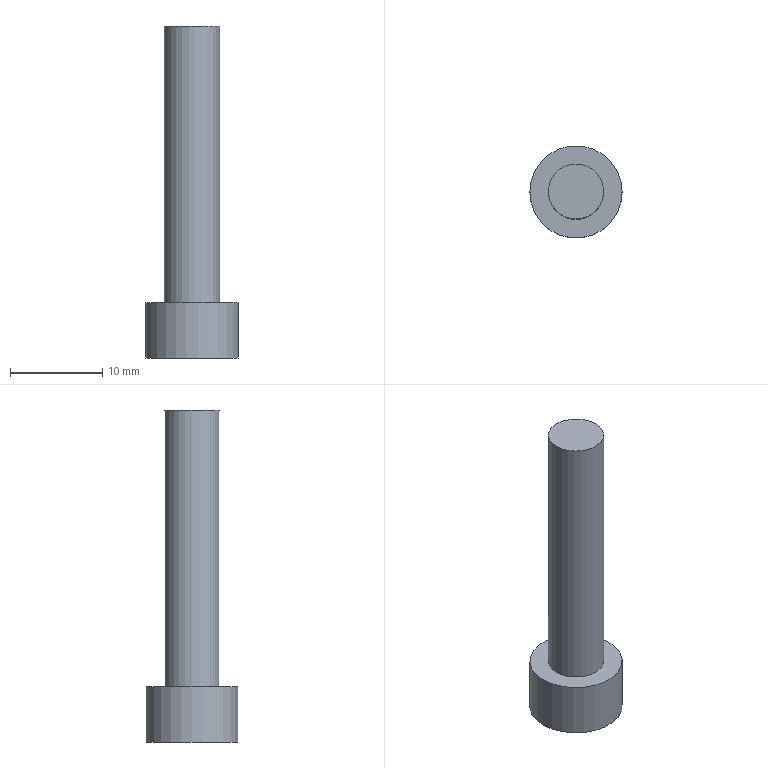Part | STEP file | 1 solid | 12 faces | box 10 x 10 x 36 mm | volume 1234 mm3 | plane 10 | cylinder 2 | commonest cylinder face diameters 6 x1 10 x1
STEP:
#1=CARTESIAN_POINT('',(0.,0.,0.));
#2=DIRECTION('',(0.,0.,1.));
#3=DIRECTION('',(1.,0.,0.));
#4=AXIS2_PLACEMENT_3D('',#1,#2,#3);
#5=CARTESIAN_POINT('',(1725.957,344.98,-64.381));
#6=VERTEX_POINT('',#5);
#7=CARTESIAN_POINT('',(1720.957,344.98,-64.381));
#8=DIRECTION('',(0.,0.,-1.));
#9=DIRECTION('',(1.,0.,0.));
#10=AXIS2_PLACEMENT_3D('',#7,#8,#9);
#11=CIRCLE('',#10,5.);
#12=CARTESIAN_POINT('',(1725.957,344.98,-64.381));
#13=DIRECTION('',(0.,0.,1.));
#14=DIRECTION('',(-1.,0.,0.));
#15=AXIS2_PLACEMENT_3D('',#12,#13,#14);
#16=PLANE('',#15);
#17=CARTESIAN_POINT('',(0.,0.));
#18=CARTESIAN_POINT('',(0.,8.66));
#19=CARTESIAN_POINT('',(7.5,4.33));
#20=CARTESIAN_POINT('',(15.,0.));
#21=CARTESIAN_POINT('',(7.5,-4.33));
#22=CARTESIAN_POINT('',(0.,-8.66));
#23=CARTESIAN_POINT('',(0.,0.));
#24=(BOUNDED_CURVE()B_SPLINE_CURVE(2,(#17,#18,#19,#20,#21,#22,#23),.UNSPECIFIED.,.T.,.F.)B_SPLINE_CURVE_WITH_KNOTS((1,2,2,2,2,1),(-2.094,0.,2.094,4.189,6.283,8.378),.UNSPECIFIED.)CURVE()GEOMETRIC_REPRESENTATION_ITEM()RATIONAL_B_SPLINE_CURVE((1.,0.5,1.,0.5,1.,0.5,1.))REPRESENTATION_ITEM(''));
#25=(GEOMETRIC_REPRESENTATION_CONTEXT(2)PARAMETRIC_REPRESENTATION_CONTEXT()REPRESENTATION_CONTEXT('',''));
#26=DEFINITIONAL_REPRESENTATION('',(#24),#25);
#27=PCURVE('',#16,#26);
#28=CARTESIAN_POINT('',(1720.957,344.98,-58.481));
#29=DIRECTION('',(0.,0.,-1.));
#30=DIRECTION('',(1.,0.,0.));
#31=AXIS2_PLACEMENT_3D('',#28,#29,#30);
#32=CYLINDRICAL_SURFACE('',#31,5.);
#33=CARTESIAN_POINT('',(0.,5.9));
#34=DIRECTION('',(1.,0.));
#35=VECTOR('',#34,1.);
#36=LINE('',#33,#35);
#37=(GEOMETRIC_REPRESENTATION_CONTEXT(2)PARAMETRIC_REPRESENTATION_CONTEXT()REPRESENTATION_CONTEXT('',''));
#38=DEFINITIONAL_REPRESENTATION('',(#36),#37);
#39=PCURVE('',#32,#38);
#40=SURFACE_CURVE('',#11,(#27,#39),.PCURVE_S1.);
#41=EDGE_CURVE('',#6,#6,#40,.T.);
#42=ORIENTED_EDGE('',*,*,#41,.T.);
#43=EDGE_LOOP('',(#42));
#44=FACE_BOUND('',#43,.T.);
#45=CARTESIAN_POINT('',(1719.514,342.48,-64.381));
#46=VERTEX_POINT('',#45);
#47=CARTESIAN_POINT('',(1722.401,342.48,-64.381));
#48=VERTEX_POINT('',#47);
#49=CARTESIAN_POINT('',(1719.514,342.48,-64.381));
#50=DIRECTION('',(1.,0.,0.));
#51=VECTOR('',#50,1.);
#52=LINE('',#49,#51);
#53=CARTESIAN_POINT('',(6.443,2.5));
#54=DIRECTION('',(-1.,0.));
#55=VECTOR('',#54,1.);
#56=LINE('',#53,#55);
#57=(GEOMETRIC_REPRESENTATION_CONTEXT(2)PARAMETRIC_REPRESENTATION_CONTEXT()REPRESENTATION_CONTEXT('',''));
#58=DEFINITIONAL_REPRESENTATION('',(#56),#57);
#59=PCURVE('',#16,#58);
#60=CARTESIAN_POINT('',(1719.514,342.48,-60.421));
#61=DIRECTION('',(0.,1.,0.));
#62=DIRECTION('',(1.,0.,0.));
#63=AXIS2_PLACEMENT_3D('',#60,#61,#62);
#64=PLANE('',#63);
#65=CARTESIAN_POINT('',(0.,3.96));
#66=DIRECTION('',(1.,0.));
#67=VECTOR('',#66,1.);
#68=LINE('',#65,#67);
#69=(GEOMETRIC_REPRESENTATION_CONTEXT(2)PARAMETRIC_REPRESENTATION_CONTEXT()REPRESENTATION_CONTEXT('',''));
#70=DEFINITIONAL_REPRESENTATION('',(#68),#69);
#71=PCURVE('',#64,#70);
#72=SURFACE_CURVE('',#52,(#59,#71),.PCURVE_S1.);
#73=EDGE_CURVE('',#46,#48,#72,.T.);
#74=ORIENTED_EDGE('',*,*,#73,.T.);
#75=CARTESIAN_POINT('',(1723.844,344.98,-64.381));
#76=VERTEX_POINT('',#75);
#77=CARTESIAN_POINT('',(1722.401,342.48,-64.381));
#78=DIRECTION('',(0.5,0.866,0.));
#79=VECTOR('',#78,1.);
#80=LINE('',#77,#79);
#81=CARTESIAN_POINT('',(3.557,2.5));
#82=DIRECTION('',(-0.5,-0.866));
#83=VECTOR('',#82,1.);
#84=LINE('',#81,#83);
#85=(GEOMETRIC_REPRESENTATION_CONTEXT(2)PARAMETRIC_REPRESENTATION_CONTEXT()REPRESENTATION_CONTEXT('',''));
#86=DEFINITIONAL_REPRESENTATION('',(#84),#85);
#87=PCURVE('',#16,#86);
#88=CARTESIAN_POINT('',(1722.401,342.48,-60.421));
#89=DIRECTION('',(-0.866,0.5,0.));
#90=DIRECTION('',(0.5,0.866,0.));
#91=AXIS2_PLACEMENT_3D('',#88,#89,#90);
#92=PLANE('',#91);
#93=CARTESIAN_POINT('',(0.,3.96));
#94=DIRECTION('',(1.,0.));
#95=VECTOR('',#94,1.);
#96=LINE('',#93,#95);
#97=(GEOMETRIC_REPRESENTATION_CONTEXT(2)PARAMETRIC_REPRESENTATION_CONTEXT()REPRESENTATION_CONTEXT('',''));
#98=DEFINITIONAL_REPRESENTATION('',(#96),#97);
#99=PCURVE('',#92,#98);
#100=SURFACE_CURVE('',#80,(#87,#99),.PCURVE_S1.);
#101=EDGE_CURVE('',#48,#76,#100,.T.);
#102=ORIENTED_EDGE('',*,*,#101,.T.);
#103=CARTESIAN_POINT('',(1722.401,347.48,-64.381));
#104=VERTEX_POINT('',#103);
#105=CARTESIAN_POINT('',(1723.844,344.98,-64.381));
#106=DIRECTION('',(-0.5,0.866,0.));
#107=VECTOR('',#106,1.);
#108=LINE('',#105,#107);
#109=CARTESIAN_POINT('',(2.113,0.));
#110=DIRECTION('',(0.5,-0.866));
#111=VECTOR('',#110,1.);
#112=LINE('',#109,#111);
#113=(GEOMETRIC_REPRESENTATION_CONTEXT(2)PARAMETRIC_REPRESENTATION_CONTEXT()REPRESENTATION_CONTEXT('',''));
#114=DEFINITIONAL_REPRESENTATION('',(#112),#113);
#115=PCURVE('',#16,#114);
#116=CARTESIAN_POINT('',(1723.844,344.98,-60.421));
#117=DIRECTION('',(-0.866,-0.5,0.));
#118=DIRECTION('',(-0.5,0.866,0.));
#119=AXIS2_PLACEMENT_3D('',#116,#117,#118);
#120=PLANE('',#119);
#121=CARTESIAN_POINT('',(0.,3.96));
#122=DIRECTION('',(1.,0.));
#123=VECTOR('',#122,1.);
#124=LINE('',#121,#123);
#125=(GEOMETRIC_REPRESENTATION_CONTEXT(2)PARAMETRIC_REPRESENTATION_CONTEXT()REPRESENTATION_CONTEXT('',''));
#126=DEFINITIONAL_REPRESENTATION('',(#124),#125);
#127=PCURVE('',#120,#126);
#128=SURFACE_CURVE('',#108,(#115,#127),.PCURVE_S1.);
#129=EDGE_CURVE('',#76,#104,#128,.T.);
#130=ORIENTED_EDGE('',*,*,#129,.T.);
#131=CARTESIAN_POINT('',(1719.514,347.48,-64.381));
#132=VERTEX_POINT('',#131);
#133=CARTESIAN_POINT('',(1722.401,347.48,-64.381));
#134=DIRECTION('',(-1.,0.,0.));
#135=VECTOR('',#134,1.);
#136=LINE('',#133,#135);
#137=CARTESIAN_POINT('',(3.557,-2.5));
#138=DIRECTION('',(1.,0.));
#139=VECTOR('',#138,1.);
#140=LINE('',#137,#139);
#141=(GEOMETRIC_REPRESENTATION_CONTEXT(2)PARAMETRIC_REPRESENTATION_CONTEXT()REPRESENTATION_CONTEXT('',''));
#142=DEFINITIONAL_REPRESENTATION('',(#140),#141);
#143=PCURVE('',#16,#142);
#144=CARTESIAN_POINT('',(1722.401,347.48,-60.421));
#145=DIRECTION('',(0.,-1.,0.));
#146=DIRECTION('',(-1.,0.,0.));
#147=AXIS2_PLACEMENT_3D('',#144,#145,#146);
#148=PLANE('',#147);
#149=CARTESIAN_POINT('',(0.,3.96));
#150=DIRECTION('',(1.,0.));
#151=VECTOR('',#150,1.);
#152=LINE('',#149,#151);
#153=(GEOMETRIC_REPRESENTATION_CONTEXT(2)PARAMETRIC_REPRESENTATION_CONTEXT()REPRESENTATION_CONTEXT('',''));
#154=DEFINITIONAL_REPRESENTATION('',(#152),#153);
#155=PCURVE('',#148,#154);
#156=SURFACE_CURVE('',#136,(#143,#155),.PCURVE_S1.);
#157=EDGE_CURVE('',#104,#132,#156,.T.);
#158=ORIENTED_EDGE('',*,*,#157,.T.);
#159=CARTESIAN_POINT('',(1718.07,344.98,-64.381));
#160=VERTEX_POINT('',#159);
#161=CARTESIAN_POINT('',(1719.514,347.48,-64.381));
#162=DIRECTION('',(-0.5,-0.866,0.));
#163=VECTOR('',#162,1.);
#164=LINE('',#161,#163);
#165=CARTESIAN_POINT('',(6.443,-2.5));
#166=DIRECTION('',(0.5,0.866));
#167=VECTOR('',#166,1.);
#168=LINE('',#165,#167);
#169=(GEOMETRIC_REPRESENTATION_CONTEXT(2)PARAMETRIC_REPRESENTATION_CONTEXT()REPRESENTATION_CONTEXT('',''));
#170=DEFINITIONAL_REPRESENTATION('',(#168),#169);
#171=PCURVE('',#16,#170);
#172=CARTESIAN_POINT('',(1719.514,347.48,-60.421));
#173=DIRECTION('',(0.866,-0.5,0.));
#174=DIRECTION('',(-0.5,-0.866,0.));
#175=AXIS2_PLACEMENT_3D('',#172,#173,#174);
#176=PLANE('',#175);
#177=CARTESIAN_POINT('',(0.,3.96));
#178=DIRECTION('',(1.,0.));
#179=VECTOR('',#178,1.);
#180=LINE('',#177,#179);
#181=(GEOMETRIC_REPRESENTATION_CONTEXT(2)PARAMETRIC_REPRESENTATION_CONTEXT()REPRESENTATION_CONTEXT('',''));
#182=DEFINITIONAL_REPRESENTATION('',(#180),#181);
#183=PCURVE('',#176,#182);
#184=SURFACE_CURVE('',#164,(#171,#183),.PCURVE_S1.);
#185=EDGE_CURVE('',#132,#160,#184,.T.);
#186=ORIENTED_EDGE('',*,*,#185,.T.);
#187=CARTESIAN_POINT('',(1718.07,344.98,-64.381));
#188=DIRECTION('',(0.5,-0.866,0.));
#189=VECTOR('',#188,1.);
#190=LINE('',#187,#189);
#191=CARTESIAN_POINT('',(7.887,0.));
#192=DIRECTION('',(-0.5,0.866));
#193=VECTOR('',#192,1.);
#194=LINE('',#191,#193);
#195=(GEOMETRIC_REPRESENTATION_CONTEXT(2)PARAMETRIC_REPRESENTATION_CONTEXT()REPRESENTATION_CONTEXT('',''));
#196=DEFINITIONAL_REPRESENTATION('',(#194),#195);
#197=PCURVE('',#16,#196);
#198=CARTESIAN_POINT('',(1718.07,344.98,-60.421));
#199=DIRECTION('',(0.866,0.5,0.));
#200=DIRECTION('',(0.5,-0.866,0.));
#201=AXIS2_PLACEMENT_3D('',#198,#199,#200);
#202=PLANE('',#201);
#203=CARTESIAN_POINT('',(0.,3.96));
#204=DIRECTION('',(1.,0.));
#205=VECTOR('',#204,1.);
#206=LINE('',#203,#205);
#207=(GEOMETRIC_REPRESENTATION_CONTEXT(2)PARAMETRIC_REPRESENTATION_CONTEXT()REPRESENTATION_CONTEXT('',''));
#208=DEFINITIONAL_REPRESENTATION('',(#206),#207);
#209=PCURVE('',#202,#208);
#210=SURFACE_CURVE('',#190,(#197,#209),.PCURVE_S1.);
#211=EDGE_CURVE('',#160,#46,#210,.T.);
#212=ORIENTED_EDGE('',*,*,#211,.T.);
#213=EDGE_LOOP('',(#74,#102,#130,#158,#186,#212));
#214=FACE_BOUND('',#213,.T.);
#215=ADVANCED_FACE('',(#44,#214),#16,.F.);
#216=ORIENTED_EDGE('',*,*,#41,.F.);
#217=CARTESIAN_POINT('',(1725.957,344.98,-58.381));
#218=VERTEX_POINT('',#217);
#219=CARTESIAN_POINT('',(1725.957,344.98,-58.381));
#220=CARTESIAN_POINT('',(1725.957,344.98,-64.381));
#221=B_SPLINE_CURVE_WITH_KNOTS('',1,(#219,#220),.UNSPECIFIED.,.F.,.F.,(2,2),(-0.1,5.9),.PIECEWISE_BEZIER_KNOTS.);
#222=CARTESIAN_POINT('',(0.,0.));
#223=DIRECTION('',(0.,1.));
#224=VECTOR('',#223,1.);
#225=LINE('',#222,#224);
#226=(GEOMETRIC_REPRESENTATION_CONTEXT(2)PARAMETRIC_REPRESENTATION_CONTEXT()REPRESENTATION_CONTEXT('',''));
#227=DEFINITIONAL_REPRESENTATION('',(#225),#226);
#228=PCURVE('',#32,#227);
#229=CARTESIAN_POINT('',(6.283,0.));
#230=DIRECTION('',(0.,1.));
#231=VECTOR('',#230,1.);
#232=LINE('',#229,#231);
#233=(GEOMETRIC_REPRESENTATION_CONTEXT(2)PARAMETRIC_REPRESENTATION_CONTEXT()REPRESENTATION_CONTEXT('',''));
#234=DEFINITIONAL_REPRESENTATION('',(#232),#233);
#235=PCURVE('',#32,#234);
#236=SEAM_CURVE('',#221,(#228,#235),.PCURVE_S1.);
#237=EDGE_CURVE('',#218,#6,#236,.T.);
#238=ORIENTED_EDGE('',*,*,#237,.F.);
#239=CARTESIAN_POINT('',(1720.957,344.98,-58.381));
#240=DIRECTION('',(0.,0.,-1.));
#241=DIRECTION('',(1.,0.,0.));
#242=AXIS2_PLACEMENT_3D('',#239,#240,#241);
#243=CIRCLE('',#242,5.);
#244=CARTESIAN_POINT('',(0.,-0.1));
#245=DIRECTION('',(1.,0.));
#246=VECTOR('',#245,1.);
#247=LINE('',#244,#246);
#248=(GEOMETRIC_REPRESENTATION_CONTEXT(2)PARAMETRIC_REPRESENTATION_CONTEXT()REPRESENTATION_CONTEXT('',''));
#249=DEFINITIONAL_REPRESENTATION('',(#247),#248);
#250=PCURVE('',#32,#249);
#251=CARTESIAN_POINT('',(1723.957,344.98,-58.381));
#252=DIRECTION('',(0.,0.,-1.));
#253=DIRECTION('',(1.,0.,0.));
#254=AXIS2_PLACEMENT_3D('',#251,#252,#253);
#255=PLANE('',#254);
#256=CARTESIAN_POINT('',(-3.,0.));
#257=DIRECTION('',(1.,0.));
#258=AXIS2_PLACEMENT_2D('',#256,#257);
#259=CIRCLE('',#258,5.);
#260=(GEOMETRIC_REPRESENTATION_CONTEXT(2)PARAMETRIC_REPRESENTATION_CONTEXT()REPRESENTATION_CONTEXT('',''));
#261=DEFINITIONAL_REPRESENTATION('',(#259),#260);
#262=PCURVE('',#255,#261);
#263=SURFACE_CURVE('',#243,(#250,#262),.PCURVE_S1.);
#264=EDGE_CURVE('',#218,#218,#263,.T.);
#265=ORIENTED_EDGE('',*,*,#264,.T.);
#266=ORIENTED_EDGE('',*,*,#237,.T.);
#267=EDGE_LOOP('',(#216,#238,#265,#266));
#268=FACE_BOUND('',#267,.T.);
#269=ADVANCED_FACE('',(#268),#32,.T.);
#270=ORIENTED_EDGE('',*,*,#264,.F.);
#271=EDGE_LOOP('',(#270));
#272=FACE_BOUND('',#271,.T.);
#273=CARTESIAN_POINT('',(1723.957,344.98,-58.381));
#274=VERTEX_POINT('',#273);
#275=CARTESIAN_POINT('',(1720.957,344.98,-58.381));
#276=DIRECTION('',(0.,0.,-1.));
#277=DIRECTION('',(1.,0.,0.));
#278=AXIS2_PLACEMENT_3D('',#275,#276,#277);
#279=CIRCLE('',#278,3.);
#280=CARTESIAN_POINT('',(-3.,0.));
#281=DIRECTION('',(1.,0.));
#282=AXIS2_PLACEMENT_2D('',#280,#281);
#283=CIRCLE('',#282,3.);
#284=(GEOMETRIC_REPRESENTATION_CONTEXT(2)PARAMETRIC_REPRESENTATION_CONTEXT()REPRESENTATION_CONTEXT('',''));
#285=DEFINITIONAL_REPRESENTATION('',(#283),#284);
#286=PCURVE('',#255,#285);
#287=CARTESIAN_POINT('',(1720.957,344.98,-58.481));
#288=DIRECTION('',(0.,0.,-1.));
#289=DIRECTION('',(1.,0.,0.));
#290=AXIS2_PLACEMENT_3D('',#287,#288,#289);
#291=CYLINDRICAL_SURFACE('',#290,3.);
#292=CARTESIAN_POINT('',(0.,-0.1));
#293=DIRECTION('',(1.,0.));
#294=VECTOR('',#293,1.);
#295=LINE('',#292,#294);
#296=(GEOMETRIC_REPRESENTATION_CONTEXT(2)PARAMETRIC_REPRESENTATION_CONTEXT()REPRESENTATION_CONTEXT('',''));
#297=DEFINITIONAL_REPRESENTATION('',(#295),#296);
#298=PCURVE('',#291,#297);
#299=SURFACE_CURVE('',#279,(#286,#298),.PCURVE_S1.);
#300=EDGE_CURVE('',#274,#274,#299,.T.);
#301=ORIENTED_EDGE('',*,*,#300,.T.);
#302=EDGE_LOOP('',(#301));
#303=FACE_BOUND('',#302,.T.);
#304=ADVANCED_FACE('',(#272,#303),#255,.F.);
#305=ORIENTED_EDGE('',*,*,#300,.F.);
#306=CARTESIAN_POINT('',(1723.957,344.98,-28.381));
#307=VERTEX_POINT('',#306);
#308=CARTESIAN_POINT('',(1723.957,344.98,-28.381));
#309=CARTESIAN_POINT('',(1723.957,344.98,-58.381));
#310=B_SPLINE_CURVE_WITH_KNOTS('',1,(#308,#309),.UNSPECIFIED.,.F.,.F.,(2,2),(-30.1,-0.1),.PIECEWISE_BEZIER_KNOTS.);
#311=CARTESIAN_POINT('',(0.,0.));
#312=DIRECTION('',(0.,1.));
#313=VECTOR('',#312,1.);
#314=LINE('',#311,#313);
#315=(GEOMETRIC_REPRESENTATION_CONTEXT(2)PARAMETRIC_REPRESENTATION_CONTEXT()REPRESENTATION_CONTEXT('',''));
#316=DEFINITIONAL_REPRESENTATION('',(#314),#315);
#317=PCURVE('',#291,#316);
#318=CARTESIAN_POINT('',(6.283,0.));
#319=DIRECTION('',(0.,1.));
#320=VECTOR('',#319,1.);
#321=LINE('',#318,#320);
#322=(GEOMETRIC_REPRESENTATION_CONTEXT(2)PARAMETRIC_REPRESENTATION_CONTEXT()REPRESENTATION_CONTEXT('',''));
#323=DEFINITIONAL_REPRESENTATION('',(#321),#322);
#324=PCURVE('',#291,#323);
#325=SEAM_CURVE('',#310,(#317,#324),.PCURVE_S1.);
#326=EDGE_CURVE('',#307,#274,#325,.T.);
#327=ORIENTED_EDGE('',*,*,#326,.F.);
#328=CARTESIAN_POINT('',(1717.957,344.98,-28.381));
#329=VERTEX_POINT('',#328);
#330=CARTESIAN_POINT('',(1720.957,344.98,-28.381));
#331=DIRECTION('',(0.,0.,-1.));
#332=DIRECTION('',(-1.,0.,0.));
#333=AXIS2_PLACEMENT_3D('',#330,#331,#332);
#334=CIRCLE('',#333,3.);
#335=CARTESIAN_POINT('',(-3.142,-30.1));
#336=DIRECTION('',(1.,0.));
#337=VECTOR('',#336,1.);
#338=LINE('',#335,#337);
#339=(GEOMETRIC_REPRESENTATION_CONTEXT(2)PARAMETRIC_REPRESENTATION_CONTEXT()REPRESENTATION_CONTEXT('',''));
#340=DEFINITIONAL_REPRESENTATION('',(#338),#339);
#341=PCURVE('',#291,#340);
#342=CARTESIAN_POINT('',(1720.957,344.98,-28.381));
#343=DIRECTION('',(0.,0.,-1.));
#344=DIRECTION('',(1.,0.,0.));
#345=AXIS2_PLACEMENT_3D('',#342,#343,#344);
#346=PLANE('',#345);
#347=CARTESIAN_POINT('',(0.,0.));
#348=DIRECTION('',(-1.,0.));
#349=AXIS2_PLACEMENT_2D('',#347,#348);
#350=CIRCLE('',#349,3.);
#351=(GEOMETRIC_REPRESENTATION_CONTEXT(2)PARAMETRIC_REPRESENTATION_CONTEXT()REPRESENTATION_CONTEXT('',''));
#352=DEFINITIONAL_REPRESENTATION('',(#350),#351);
#353=PCURVE('',#346,#352);
#354=SURFACE_CURVE('',#334,(#341,#353),.PCURVE_S1.);
#355=EDGE_CURVE('',#307,#329,#354,.T.);
#356=ORIENTED_EDGE('',*,*,#355,.T.);
#357=CARTESIAN_POINT('',(1720.957,344.98,-28.381));
#358=DIRECTION('',(0.,0.,-1.));
#359=DIRECTION('',(-1.,0.,0.));
#360=AXIS2_PLACEMENT_3D('',#357,#358,#359);
#361=CIRCLE('',#360,3.);
#362=CARTESIAN_POINT('',(3.142,-30.1));
#363=DIRECTION('',(1.,0.));
#364=VECTOR('',#363,1.);
#365=LINE('',#362,#364);
#366=(GEOMETRIC_REPRESENTATION_CONTEXT(2)PARAMETRIC_REPRESENTATION_CONTEXT()REPRESENTATION_CONTEXT('',''));
#367=DEFINITIONAL_REPRESENTATION('',(#365),#366);
#368=PCURVE('',#291,#367);
#369=CARTESIAN_POINT('',(0.,0.));
#370=DIRECTION('',(-1.,0.));
#371=AXIS2_PLACEMENT_2D('',#369,#370);
#372=CIRCLE('',#371,3.);
#373=(GEOMETRIC_REPRESENTATION_CONTEXT(2)PARAMETRIC_REPRESENTATION_CONTEXT()REPRESENTATION_CONTEXT('',''));
#374=DEFINITIONAL_REPRESENTATION('',(#372),#373);
#375=PCURVE('',#346,#374);
#376=SURFACE_CURVE('',#361,(#368,#375),.PCURVE_S1.);
#377=EDGE_CURVE('',#329,#307,#376,.T.);
#378=ORIENTED_EDGE('',*,*,#377,.T.);
#379=ORIENTED_EDGE('',*,*,#326,.T.);
#380=EDGE_LOOP('',(#305,#327,#356,#378,#379));
#381=FACE_BOUND('',#380,.T.);
#382=ADVANCED_FACE('',(#381),#291,.T.);
#383=ORIENTED_EDGE('',*,*,#377,.F.);
#384=ORIENTED_EDGE('',*,*,#355,.F.);
#385=EDGE_LOOP('',(#383,#384));
#386=FACE_BOUND('',#385,.T.);
#387=ADVANCED_FACE('',(#386),#346,.F.);
#388=ORIENTED_EDGE('',*,*,#73,.F.);
#389=CARTESIAN_POINT('',(1719.514,342.48,-60.421));
#390=VERTEX_POINT('',#389);
#391=CARTESIAN_POINT('',(1719.514,342.48,-60.421));
#392=DIRECTION('',(0.,0.,1.));
#393=VECTOR('',#392,1.);
#394=LINE('',#391,#393);
#395=CARTESIAN_POINT('',(0.,0.));
#396=DIRECTION('',(0.,-1.));
#397=VECTOR('',#396,1.);
#398=LINE('',#395,#397);
#399=(GEOMETRIC_REPRESENTATION_CONTEXT(2)PARAMETRIC_REPRESENTATION_CONTEXT()REPRESENTATION_CONTEXT('',''));
#400=DEFINITIONAL_REPRESENTATION('',(#398),#399);
#401=PCURVE('',#64,#400);
#402=CARTESIAN_POINT('',(2.887,0.));
#403=DIRECTION('',(0.,-1.));
#404=VECTOR('',#403,1.);
#405=LINE('',#402,#404);
#406=(GEOMETRIC_REPRESENTATION_CONTEXT(2)PARAMETRIC_REPRESENTATION_CONTEXT()REPRESENTATION_CONTEXT('',''));
#407=DEFINITIONAL_REPRESENTATION('',(#405),#406);
#408=PCURVE('',#202,#407);
#409=SURFACE_CURVE('',#394,(#401,#408),.PCURVE_S1.);
#410=EDGE_CURVE('',#46,#390,#409,.T.);
#411=ORIENTED_EDGE('',*,*,#410,.T.);
#412=CARTESIAN_POINT('',(1722.401,342.48,-60.421));
#413=VERTEX_POINT('',#412);
#414=CARTESIAN_POINT('',(1719.514,342.48,-60.421));
#415=DIRECTION('',(-1.,0.,0.));
#416=VECTOR('',#415,1.);
#417=LINE('',#414,#416);
#418=CARTESIAN_POINT('',(0.,0.));
#419=DIRECTION('',(-1.,0.));
#420=VECTOR('',#419,1.);
#421=LINE('',#418,#420);
#422=(GEOMETRIC_REPRESENTATION_CONTEXT(2)PARAMETRIC_REPRESENTATION_CONTEXT()REPRESENTATION_CONTEXT('',''));
#423=DEFINITIONAL_REPRESENTATION('',(#421),#422);
#424=PCURVE('',#64,#423);
#425=CARTESIAN_POINT('',(1720.957,344.98,-60.421));
#426=DIRECTION('',(0.,0.,1.));
#427=DIRECTION('',(-1.,0.,0.));
#428=AXIS2_PLACEMENT_3D('',#425,#426,#427);
#429=PLANE('',#428);
#430=CARTESIAN_POINT('',(1.443,2.5));
#431=DIRECTION('',(1.,0.));
#432=VECTOR('',#431,1.);
#433=LINE('',#430,#432);
#434=(GEOMETRIC_REPRESENTATION_CONTEXT(2)PARAMETRIC_REPRESENTATION_CONTEXT()REPRESENTATION_CONTEXT('',''));
#435=DEFINITIONAL_REPRESENTATION('',(#433),#434);
#436=PCURVE('',#429,#435);
#437=SURFACE_CURVE('',#417,(#424,#436),.PCURVE_S1.);
#438=EDGE_CURVE('',#413,#390,#437,.T.);
#439=ORIENTED_EDGE('',*,*,#438,.F.);
#440=CARTESIAN_POINT('',(1722.401,342.48,-60.421));
#441=DIRECTION('',(0.,0.,1.));
#442=VECTOR('',#441,1.);
#443=LINE('',#440,#442);
#444=CARTESIAN_POINT('',(2.887,0.));
#445=DIRECTION('',(0.,-1.));
#446=VECTOR('',#445,1.);
#447=LINE('',#444,#446);
#448=(GEOMETRIC_REPRESENTATION_CONTEXT(2)PARAMETRIC_REPRESENTATION_CONTEXT()REPRESENTATION_CONTEXT('',''));
#449=DEFINITIONAL_REPRESENTATION('',(#447),#448);
#450=PCURVE('',#64,#449);
#451=CARTESIAN_POINT('',(0.,0.));
#452=DIRECTION('',(0.,-1.));
#453=VECTOR('',#452,1.);
#454=LINE('',#451,#453);
#455=(GEOMETRIC_REPRESENTATION_CONTEXT(2)PARAMETRIC_REPRESENTATION_CONTEXT()REPRESENTATION_CONTEXT('',''));
#456=DEFINITIONAL_REPRESENTATION('',(#454),#455);
#457=PCURVE('',#92,#456);
#458=SURFACE_CURVE('',#443,(#450,#457),.PCURVE_S1.);
#459=EDGE_CURVE('',#48,#413,#458,.T.);
#460=ORIENTED_EDGE('',*,*,#459,.F.);
#461=EDGE_LOOP('',(#388,#411,#439,#460));
#462=FACE_BOUND('',#461,.T.);
#463=ADVANCED_FACE('',(#462),#64,.T.);
#464=ORIENTED_EDGE('',*,*,#101,.F.);
#465=ORIENTED_EDGE('',*,*,#459,.T.);
#466=CARTESIAN_POINT('',(1723.844,344.98,-60.421));
#467=VERTEX_POINT('',#466);
#468=CARTESIAN_POINT('',(1722.401,342.48,-60.421));
#469=DIRECTION('',(-0.5,-0.866,0.));
#470=VECTOR('',#469,1.);
#471=LINE('',#468,#470);
#472=CARTESIAN_POINT('',(0.,0.));
#473=DIRECTION('',(-1.,0.));
#474=VECTOR('',#473,1.);
#475=LINE('',#472,#474);
#476=(GEOMETRIC_REPRESENTATION_CONTEXT(2)PARAMETRIC_REPRESENTATION_CONTEXT()REPRESENTATION_CONTEXT('',''));
#477=DEFINITIONAL_REPRESENTATION('',(#475),#476);
#478=PCURVE('',#92,#477);
#479=CARTESIAN_POINT('',(-1.443,2.5));
#480=DIRECTION('',(0.5,0.866));
#481=VECTOR('',#480,1.);
#482=LINE('',#479,#481);
#483=(GEOMETRIC_REPRESENTATION_CONTEXT(2)PARAMETRIC_REPRESENTATION_CONTEXT()REPRESENTATION_CONTEXT('',''));
#484=DEFINITIONAL_REPRESENTATION('',(#482),#483);
#485=PCURVE('',#429,#484);
#486=SURFACE_CURVE('',#471,(#478,#485),.PCURVE_S1.);
#487=EDGE_CURVE('',#467,#413,#486,.T.);
#488=ORIENTED_EDGE('',*,*,#487,.F.);
#489=CARTESIAN_POINT('',(1723.844,344.98,-60.421));
#490=DIRECTION('',(0.,0.,1.));
#491=VECTOR('',#490,1.);
#492=LINE('',#489,#491);
#493=CARTESIAN_POINT('',(2.887,0.));
#494=DIRECTION('',(0.,-1.));
#495=VECTOR('',#494,1.);
#496=LINE('',#493,#495);
#497=(GEOMETRIC_REPRESENTATION_CONTEXT(2)PARAMETRIC_REPRESENTATION_CONTEXT()REPRESENTATION_CONTEXT('',''));
#498=DEFINITIONAL_REPRESENTATION('',(#496),#497);
#499=PCURVE('',#92,#498);
#500=CARTESIAN_POINT('',(0.,0.));
#501=DIRECTION('',(0.,-1.));
#502=VECTOR('',#501,1.);
#503=LINE('',#500,#502);
#504=(GEOMETRIC_REPRESENTATION_CONTEXT(2)PARAMETRIC_REPRESENTATION_CONTEXT()REPRESENTATION_CONTEXT('',''));
#505=DEFINITIONAL_REPRESENTATION('',(#503),#504);
#506=PCURVE('',#120,#505);
#507=SURFACE_CURVE('',#492,(#499,#506),.PCURVE_S1.);
#508=EDGE_CURVE('',#76,#467,#507,.T.);
#509=ORIENTED_EDGE('',*,*,#508,.F.);
#510=EDGE_LOOP('',(#464,#465,#488,#509));
#511=FACE_BOUND('',#510,.T.);
#512=ADVANCED_FACE('',(#511),#92,.T.);
#513=ORIENTED_EDGE('',*,*,#129,.F.);
#514=ORIENTED_EDGE('',*,*,#508,.T.);
#515=CARTESIAN_POINT('',(1722.401,347.48,-60.421));
#516=VERTEX_POINT('',#515);
#517=CARTESIAN_POINT('',(1723.844,344.98,-60.421));
#518=DIRECTION('',(0.5,-0.866,0.));
#519=VECTOR('',#518,1.);
#520=LINE('',#517,#519);
#521=CARTESIAN_POINT('',(0.,0.));
#522=DIRECTION('',(-1.,0.));
#523=VECTOR('',#522,1.);
#524=LINE('',#521,#523);
#525=(GEOMETRIC_REPRESENTATION_CONTEXT(2)PARAMETRIC_REPRESENTATION_CONTEXT()REPRESENTATION_CONTEXT('',''));
#526=DEFINITIONAL_REPRESENTATION('',(#524),#525);
#527=PCURVE('',#120,#526);
#528=CARTESIAN_POINT('',(-2.887,0.));
#529=DIRECTION('',(-0.5,0.866));
#530=VECTOR('',#529,1.);
#531=LINE('',#528,#530);
#532=(GEOMETRIC_REPRESENTATION_CONTEXT(2)PARAMETRIC_REPRESENTATION_CONTEXT()REPRESENTATION_CONTEXT('',''));
#533=DEFINITIONAL_REPRESENTATION('',(#531),#532);
#534=PCURVE('',#429,#533);
#535=SURFACE_CURVE('',#520,(#527,#534),.PCURVE_S1.);
#536=EDGE_CURVE('',#516,#467,#535,.T.);
#537=ORIENTED_EDGE('',*,*,#536,.F.);
#538=CARTESIAN_POINT('',(1722.401,347.48,-60.421));
#539=DIRECTION('',(0.,0.,1.));
#540=VECTOR('',#539,1.);
#541=LINE('',#538,#540);
#542=CARTESIAN_POINT('',(2.887,0.));
#543=DIRECTION('',(0.,-1.));
#544=VECTOR('',#543,1.);
#545=LINE('',#542,#544);
#546=(GEOMETRIC_REPRESENTATION_CONTEXT(2)PARAMETRIC_REPRESENTATION_CONTEXT()REPRESENTATION_CONTEXT('',''));
#547=DEFINITIONAL_REPRESENTATION('',(#545),#546);
#548=PCURVE('',#120,#547);
#549=CARTESIAN_POINT('',(0.,0.));
#550=DIRECTION('',(0.,-1.));
#551=VECTOR('',#550,1.);
#552=LINE('',#549,#551);
#553=(GEOMETRIC_REPRESENTATION_CONTEXT(2)PARAMETRIC_REPRESENTATION_CONTEXT()REPRESENTATION_CONTEXT('',''));
#554=DEFINITIONAL_REPRESENTATION('',(#552),#553);
#555=PCURVE('',#148,#554);
#556=SURFACE_CURVE('',#541,(#548,#555),.PCURVE_S1.);
#557=EDGE_CURVE('',#104,#516,#556,.T.);
#558=ORIENTED_EDGE('',*,*,#557,.F.);
#559=EDGE_LOOP('',(#513,#514,#537,#558));
#560=FACE_BOUND('',#559,.T.);
#561=ADVANCED_FACE('',(#560),#120,.T.);
#562=ORIENTED_EDGE('',*,*,#157,.F.);
#563=ORIENTED_EDGE('',*,*,#557,.T.);
#564=CARTESIAN_POINT('',(1719.514,347.48,-60.421));
#565=VERTEX_POINT('',#564);
#566=CARTESIAN_POINT('',(1722.401,347.48,-60.421));
#567=DIRECTION('',(1.,0.,0.));
#568=VECTOR('',#567,1.);
#569=LINE('',#566,#568);
#570=CARTESIAN_POINT('',(0.,0.));
#571=DIRECTION('',(-1.,0.));
#572=VECTOR('',#571,1.);
#573=LINE('',#570,#572);
#574=(GEOMETRIC_REPRESENTATION_CONTEXT(2)PARAMETRIC_REPRESENTATION_CONTEXT()REPRESENTATION_CONTEXT('',''));
#575=DEFINITIONAL_REPRESENTATION('',(#573),#574);
#576=PCURVE('',#148,#575);
#577=CARTESIAN_POINT('',(-1.443,-2.5));
#578=DIRECTION('',(-1.,0.));
#579=VECTOR('',#578,1.);
#580=LINE('',#577,#579);
#581=(GEOMETRIC_REPRESENTATION_CONTEXT(2)PARAMETRIC_REPRESENTATION_CONTEXT()REPRESENTATION_CONTEXT('',''));
#582=DEFINITIONAL_REPRESENTATION('',(#580),#581);
#583=PCURVE('',#429,#582);
#584=SURFACE_CURVE('',#569,(#576,#583),.PCURVE_S1.);
#585=EDGE_CURVE('',#565,#516,#584,.T.);
#586=ORIENTED_EDGE('',*,*,#585,.F.);
#587=CARTESIAN_POINT('',(1719.514,347.48,-60.421));
#588=DIRECTION('',(0.,0.,1.));
#589=VECTOR('',#588,1.);
#590=LINE('',#587,#589);
#591=CARTESIAN_POINT('',(2.887,0.));
#592=DIRECTION('',(0.,-1.));
#593=VECTOR('',#592,1.);
#594=LINE('',#591,#593);
#595=(GEOMETRIC_REPRESENTATION_CONTEXT(2)PARAMETRIC_REPRESENTATION_CONTEXT()REPRESENTATION_CONTEXT('',''));
#596=DEFINITIONAL_REPRESENTATION('',(#594),#595);
#597=PCURVE('',#148,#596);
#598=CARTESIAN_POINT('',(0.,0.));
#599=DIRECTION('',(0.,-1.));
#600=VECTOR('',#599,1.);
#601=LINE('',#598,#600);
#602=(GEOMETRIC_REPRESENTATION_CONTEXT(2)PARAMETRIC_REPRESENTATION_CONTEXT()REPRESENTATION_CONTEXT('',''));
#603=DEFINITIONAL_REPRESENTATION('',(#601),#602);
#604=PCURVE('',#176,#603);
#605=SURFACE_CURVE('',#590,(#597,#604),.PCURVE_S1.);
#606=EDGE_CURVE('',#132,#565,#605,.T.);
#607=ORIENTED_EDGE('',*,*,#606,.F.);
#608=EDGE_LOOP('',(#562,#563,#586,#607));
#609=FACE_BOUND('',#608,.T.);
#610=ADVANCED_FACE('',(#609),#148,.T.);
#611=ORIENTED_EDGE('',*,*,#185,.F.);
#612=ORIENTED_EDGE('',*,*,#606,.T.);
#613=CARTESIAN_POINT('',(1718.07,344.98,-60.421));
#614=VERTEX_POINT('',#613);
#615=CARTESIAN_POINT('',(1719.514,347.48,-60.421));
#616=DIRECTION('',(0.5,0.866,0.));
#617=VECTOR('',#616,1.);
#618=LINE('',#615,#617);
#619=CARTESIAN_POINT('',(0.,0.));
#620=DIRECTION('',(-1.,0.));
#621=VECTOR('',#620,1.);
#622=LINE('',#619,#621);
#623=(GEOMETRIC_REPRESENTATION_CONTEXT(2)PARAMETRIC_REPRESENTATION_CONTEXT()REPRESENTATION_CONTEXT('',''));
#624=DEFINITIONAL_REPRESENTATION('',(#622),#623);
#625=PCURVE('',#176,#624);
#626=CARTESIAN_POINT('',(1.443,-2.5));
#627=DIRECTION('',(-0.5,-0.866));
#628=VECTOR('',#627,1.);
#629=LINE('',#626,#628);
#630=(GEOMETRIC_REPRESENTATION_CONTEXT(2)PARAMETRIC_REPRESENTATION_CONTEXT()REPRESENTATION_CONTEXT('',''));
#631=DEFINITIONAL_REPRESENTATION('',(#629),#630);
#632=PCURVE('',#429,#631);
#633=SURFACE_CURVE('',#618,(#625,#632),.PCURVE_S1.);
#634=EDGE_CURVE('',#614,#565,#633,.T.);
#635=ORIENTED_EDGE('',*,*,#634,.F.);
#636=CARTESIAN_POINT('',(1718.07,344.98,-60.421));
#637=DIRECTION('',(0.,0.,1.));
#638=VECTOR('',#637,1.);
#639=LINE('',#636,#638);
#640=CARTESIAN_POINT('',(2.887,0.));
#641=DIRECTION('',(0.,-1.));
#642=VECTOR('',#641,1.);
#643=LINE('',#640,#642);
#644=(GEOMETRIC_REPRESENTATION_CONTEXT(2)PARAMETRIC_REPRESENTATION_CONTEXT()REPRESENTATION_CONTEXT('',''));
#645=DEFINITIONAL_REPRESENTATION('',(#643),#644);
#646=PCURVE('',#176,#645);
#647=CARTESIAN_POINT('',(0.,0.));
#648=DIRECTION('',(0.,-1.));
#649=VECTOR('',#648,1.);
#650=LINE('',#647,#649);
#651=(GEOMETRIC_REPRESENTATION_CONTEXT(2)PARAMETRIC_REPRESENTATION_CONTEXT()REPRESENTATION_CONTEXT('',''));
#652=DEFINITIONAL_REPRESENTATION('',(#650),#651);
#653=PCURVE('',#202,#652);
#654=SURFACE_CURVE('',#639,(#646,#653),.PCURVE_S1.);
#655=EDGE_CURVE('',#160,#614,#654,.T.);
#656=ORIENTED_EDGE('',*,*,#655,.F.);
#657=EDGE_LOOP('',(#611,#612,#635,#656));
#658=FACE_BOUND('',#657,.T.);
#659=ADVANCED_FACE('',(#658),#176,.T.);
#660=ORIENTED_EDGE('',*,*,#211,.F.);
#661=ORIENTED_EDGE('',*,*,#655,.T.);
#662=CARTESIAN_POINT('',(1718.07,344.98,-60.421));
#663=DIRECTION('',(-0.5,0.866,0.));
#664=VECTOR('',#663,1.);
#665=LINE('',#662,#664);
#666=CARTESIAN_POINT('',(0.,0.));
#667=DIRECTION('',(-1.,0.));
#668=VECTOR('',#667,1.);
#669=LINE('',#666,#668);
#670=(GEOMETRIC_REPRESENTATION_CONTEXT(2)PARAMETRIC_REPRESENTATION_CONTEXT()REPRESENTATION_CONTEXT('',''));
#671=DEFINITIONAL_REPRESENTATION('',(#669),#670);
#672=PCURVE('',#202,#671);
#673=CARTESIAN_POINT('',(2.887,0.));
#674=DIRECTION('',(0.5,-0.866));
#675=VECTOR('',#674,1.);
#676=LINE('',#673,#675);
#677=(GEOMETRIC_REPRESENTATION_CONTEXT(2)PARAMETRIC_REPRESENTATION_CONTEXT()REPRESENTATION_CONTEXT('',''));
#678=DEFINITIONAL_REPRESENTATION('',(#676),#677);
#679=PCURVE('',#429,#678);
#680=SURFACE_CURVE('',#665,(#672,#679),.PCURVE_S1.);
#681=EDGE_CURVE('',#390,#614,#680,.T.);
#682=ORIENTED_EDGE('',*,*,#681,.F.);
#683=ORIENTED_EDGE('',*,*,#410,.F.);
#684=EDGE_LOOP('',(#660,#661,#682,#683));
#685=FACE_BOUND('',#684,.T.);
#686=ADVANCED_FACE('',(#685),#202,.T.);
#687=ORIENTED_EDGE('',*,*,#438,.T.);
#688=ORIENTED_EDGE('',*,*,#681,.T.);
#689=ORIENTED_EDGE('',*,*,#634,.T.);
#690=ORIENTED_EDGE('',*,*,#585,.T.);
#691=ORIENTED_EDGE('',*,*,#536,.T.);
#692=ORIENTED_EDGE('',*,*,#487,.T.);
#693=EDGE_LOOP('',(#687,#688,#689,#690,#691,#692));
#694=FACE_BOUND('',#693,.T.);
#695=ADVANCED_FACE('',(#694),#429,.F.);
#696=CLOSED_SHELL('',(#215,#269,#304,#382,#387,#463,#512,#561,#610,#659,#686,#695));
#697=MANIFOLD_SOLID_BREP('',#696);
#698=(LENGTH_UNIT()NAMED_UNIT(*)SI_UNIT(.MILLI.,.METRE.));
#699=UNCERTAINTY_MEASURE_WITH_UNIT(LENGTH_MEASURE(0.000002),#698,'','');
#700=(NAMED_UNIT(*)PLANE_ANGLE_UNIT()SI_UNIT($,.RADIAN.));
#701=(NAMED_UNIT(*)SI_UNIT($,.STERADIAN.)SOLID_ANGLE_UNIT());
#702=(GEOMETRIC_REPRESENTATION_CONTEXT(3)GLOBAL_UNCERTAINTY_ASSIGNED_CONTEXT((#699))GLOBAL_UNIT_ASSIGNED_CONTEXT((#698,#700,#701))REPRESENTATION_CONTEXT('',''));
#703=ADVANCED_BREP_SHAPE_REPRESENTATION('',(#4,#697),#702);